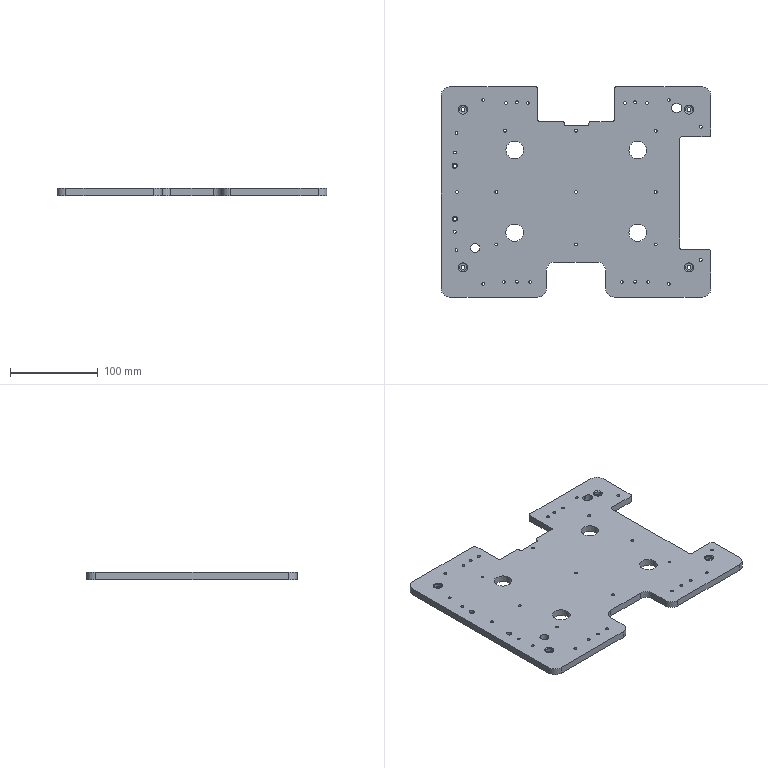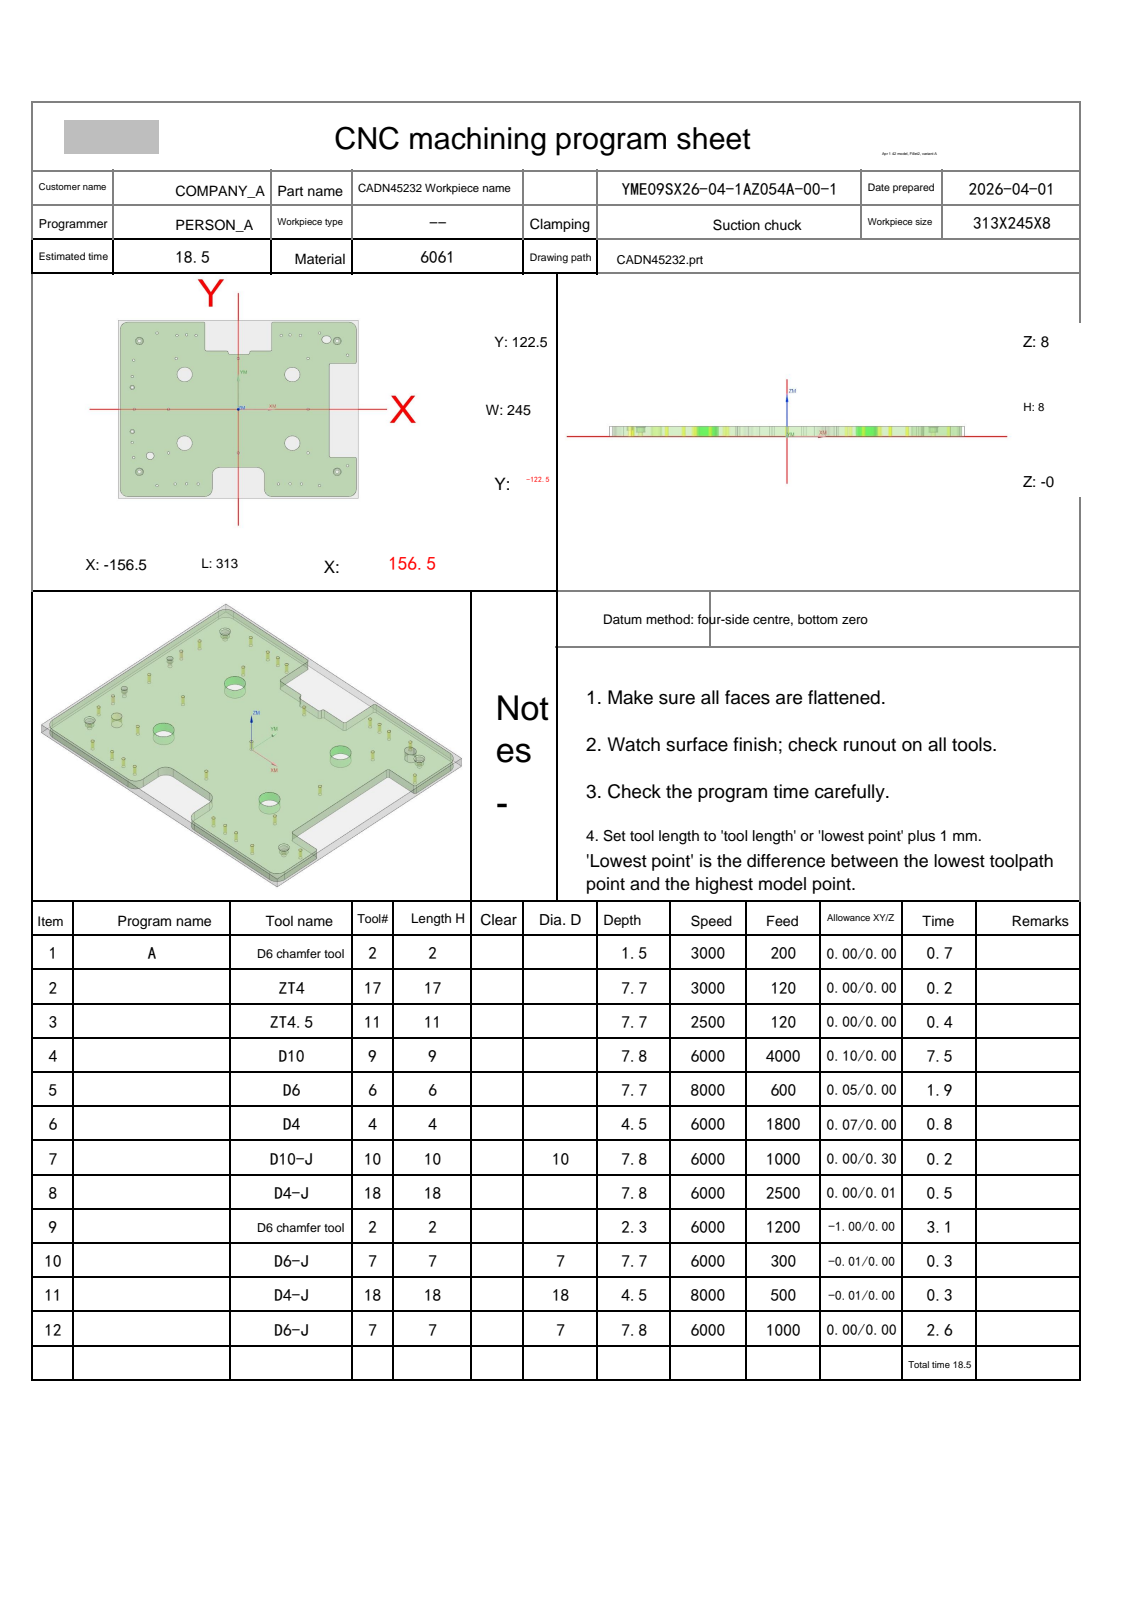NC program | NX | posted by the shop | part box 308 x 240 x 8 mm
Lines 6151 to 6786 of 6786:
N9 T02 M06
(D6 chamfer tool  D=6. R=0. H=02 ce=0.00 di=0.00)
G00 G90 G54 X-156.128 Y-.25 M03 S6000
G43 H02 Z28.
M08
Z10.099
G01 Z6.501 F1200.
G03 X-155.828 Y-.33 I.3 J.52
X-155.308 Y-.03 I0.0 J.6
G01 X-155.3 Y0.0
Y110.
G02 X-144. Y121.3 I11.3 J0.0
G01 X-45.5
G02 X-42.2 Y118. I0.0 J-3.3
G01 Y82.355
X-42.178 Y82.137
X-42.117 Y81.965
X-42.002 Y81.806
X-41.848 Y81.685
X-41.666 Y81.612
X-41.435 Y81.589
X-15.216
X-15.151 Y81.587
X-15.087 Y81.582
X-14.647 Y81.538
X-14.491 Y81.513
X-14.34 Y81.469
X-13.846 Y81.293
X-13.678 Y81.219
X-13.522 Y81.123
X-13.063 Y80.793
X-12.923 Y80.675
X-12.8 Y80.539
X-12.451 Y80.094
X-12.349 Y79.942
X-12.269 Y79.777
X-12.058 Y79.253
X-12.002 Y79.078
G02 X-11.909 Y78.005 I-6.16 J-1.074
X-11.916 Y77.706 I-6.252 J0.0
G03 X-11.216 Y77.006 I.7 J0.0
G01 X12.784
G03 X13.484 Y77.706 I0.0 J.7
G02 X13.476 Y78.014 I5.995 J.309
X13.559 Y79.013 I6.003 J0.0
G01 X13.603 Y79.164
X13.779 Y79.659
X13.853 Y79.827
X13.949 Y79.983
X14.28 Y80.441
X14.397 Y80.582
X14.533 Y80.705
X14.978 Y81.053
X15.13 Y81.156
X15.295 Y81.236
X15.819 Y81.447
X15.994 Y81.503
X16.174 Y81.534
X16.654 Y81.582
X16.719 Y81.587
X16.784 Y81.589
X41.435
X41.652 Y81.611
X41.824 Y81.672
X41.983 Y81.786
X42.104 Y81.941
X42.177 Y82.123
X42.2 Y82.355
Y118.
G02 X45.5 Y121.3 I3.3 J0.0
G01 X144.
G02 X155.3 Y110. I0.0 J-11.3
G01 Y65.004
G02 X152. Y61.704 I-3.3 J0.0
G01 X120.728
X120.511 Y61.682
X120.339 Y61.621
X120.18 Y61.506
X120.059 Y61.352
X119.986 Y61.17
X119.963 Y60.939
Y-63.931
X119.984 Y-64.149
X120.046 Y-64.32
X120.16 Y-64.479
X120.315 Y-64.6
X120.497 Y-64.673
X120.728 Y-64.696
X152.
G02 X155.3 Y-67.996 I0.0 J-3.3
G01 Y-110.
G02 X144. Y-121.3 I-11.3 J0.0
G01 X44.
G02 X32.7 Y-110. I0.0 J11.3
G01 Y-90.
G03 X24. Y-81.3 I-8.7 J0.0
G01 X-24.
G03 X-32.7 Y-90. I0.0 J-8.7
G01 Y-110.
G02 X-44. Y-121.3 I-11.3 J0.0
G01 X-144.
G02 X-155.3 Y-110. I0.0 J11.3
G01 Y0.0
X-155.308 Y.03
G03 X-155.828 Y.33 I-.52 J-.3
X-156.128 Y.25 I0.0 J-.6
G01 Z10.099
G00 Z28.
X-77.885 Y48.289
Z10.119
G01 Z6.501
G03 X-78.16 Y48.355 I-.275 J-.533
X-78.693 Y48.03 I0.0 J-.6
G01 X-78.7 Y48.
G03 X-70. Y39.3 I8.7 J0.0
X-61.3 Y48. I0.0 J8.7
X-70. Y56.7 I-8.7 J0.0
X-78.7 Y48. I0.0 J-8.7
G01 X-78.693 Y47.97
G03 X-78.16 Y47.645 I.533 J.275
X-77.885 Y47.711 I0.0 J.6
G01 Z10.119
G00 Z28.
X-77.99 Y-46.278
Z10.119
G01 Z6.501
G03 X-78.265 Y-46.211 I-.275 J-.533
X-78.798 Y-46.536 I0.0 J-.6
G01 X-78.805 Y-46.566
G03 X-70.105 Y-55.266 I8.7 J0.0
X-61.405 Y-46.566 I0.0 J8.7
X-70.105 Y-37.866 I-8.7 J0.0
X-78.805 Y-46.566 I0.0 J-8.7
G01 X-78.798 Y-46.597
G03 X-78.265 Y-46.922 I.533 J.275
X-77.99 Y-46.855 I0.0 J.6
G01 Z10.119
G00 Z28.
X62.573 Y-46.278
Z10.119
G01 Z6.501
G03 X62.298 Y-46.211 I-.275 J-.533
X61.765 Y-46.536 I0.0 J-.6
G01 X61.758 Y-46.566
G03 X70.458 Y-55.266 I8.7 J0.0
X79.158 Y-46.566 I0.0 J8.7
X70.458 Y-37.866 I-8.7 J0.0
X61.758 Y-46.566 I0.0 J-8.7
G01 X61.765 Y-46.597
G03 X62.298 Y-46.922 I.533 J.275
X62.573 Y-46.855 I0.0 J.6
G01 Z10.119
G00 Z28.
Y48.135
Z10.119
G01 Z6.501
G03 X62.298 Y48.202 I-.275 J-.533
X61.765 Y47.877 I0.0 J-.6
G01 X61.758 Y47.847
G03 X70.458 Y39.147 I8.7 J0.0
X79.158 Y47.847 I0.0 J8.7
X70.458 Y56.547 I-8.7 J0.0
X61.758 Y47.847 I0.0 J-8.7
G01 X61.765 Y47.816
G03 X62.298 Y47.491 I.533 J.275
X62.573 Y47.558 I0.0 J.6
G01 Z10.119
G00 Z28.
X114.75 Y93.136
Z10.099
G01 Z6.501
G03 X114.67 Y92.836 I.52 J-.3
X114.97 Y92.317 I.6 J0.0
G01 X115. Y92.309
X116.
G03 X119.7 Y96.009 I0.0 J3.7
X116. Y99.709 I-3.7 J0.0
G01 X114.
G03 X110.3 Y96.009 I0.0 J-3.7
X114. Y92.309 I3.7 J0.0
G01 X115.
X115.03 Y92.317
G03 X115.33 Y92.836 I-.3 J.52
X115.25 Y93.136 I-.6 J0.0
G01 Z10.099
G00 Z28.
G00 G90 X0.0 Y0.0 M03 S5000
Z28.
G98 G81 X0.0 Y0.0 Z5.8 R11. F150.
Y-60.
X-52.35 Y-102.765
X-67.5 Y-102.5
X-82.35 Y-102.765
X-106. Y-105.
X-136.5 Y-66.5
X-138.327 Y-45.597
X-91. Y-60.
Y0.0
X-135.8
X-138.327 Y45.083
X-136.5 Y67.5
X-106. Y105.
X-81. Y70.
X-80. Y101.6
X-67.5 Y102.5
X-55. Y101.6
X0.0 Y70.
X56. Y101.6
X67.5 Y102.5
X81. Y101.6
X106. Y105.
X142.5 Y74.508
X91. Y70.
Y0.0
Y-60.
X142.5 Y-77.5
X106. Y-105.
X82.35 Y-102.765
X67.5 Y-102.5
X52.35 Y-102.765
G80
G00 Z28.
G00 G90 X-138.239 Y29.77 M03 S6000
Z28.
Z6.5
G01 Z6. F600.
X-138.103 Y29.755
X-137.947 Y29.747
G03 X-137.002 Y30.083 I0.0 J1.5
X-138.327 Y31.408 I-1.325 J0.0
X-139.652 Y30.083 I0.0 J-1.325
X-138.327 Y28.758 I1.325 J0.0
X-137.002 Y30.083 I0.0 J1.325
X-137.947 Y30.418 I-.945 J-1.165
G01 X-138.103 Y30.41
X-138.239 Y30.396
Z6.5
G00 Z28.
Y-30.91
Z6.5
G01 Z6.
X-138.103 Y-30.925
X-137.947 Y-30.933
G03 X-137.002 Y-30.597 I0.0 J1.5
X-138.327 Y-29.272 I-1.325 J0.0
X-139.652 Y-30.597 I0.0 J-1.325
X-138.327 Y-31.922 I1.325 J0.0
X-137.002 Y-30.597 I0.0 J1.325
X-137.947 Y-30.262 I-.945 J-1.165
G01 X-138.103 Y-30.27
X-138.239 Y-30.284
Z6.5
G00 Z28.
G00 G90 X-129.667 Y96.677 M03 S6000
Z28.
Z7.
G01 Z6.5 F600.
X-129.75 Y97.009
G03 X-132.75 Y94.009 I0.0 J-3.
X-129. Y90.259 I3.75 J0.0
X-125.25 Y94.009 I0.0 J3.75
X-129. Y97.759 I-3.75 J0.0
X-132.75 Y94.009 I0.0 J-3.75
X-129.75 Y91.009 I3. J0.0
G01 X-129.667 Y91.341
Z7.
G00 Z28.
Y-83.323
Z7.
G01 Z6.5
X-129.75 Y-82.991
G03 X-132.75 Y-85.991 I0.0 J-3.
X-129. Y-89.741 I3.75 J0.0
X-125.25 Y-85.991 I0.0 J3.75
X-129. Y-82.241 I-3.75 J0.0
X-132.75 Y-85.991 I0.0 J-3.75
X-129.75 Y-88.991 I3. J0.0
G01 X-129.667 Y-88.659
Z7.
G00 Z28.
X128.333 Y-83.323
Z7.
G01 Z6.5
X128.25 Y-82.991
G03 X125.25 Y-85.991 I0.0 J-3.
X129. Y-89.741 I3.75 J0.0
X132.75 Y-85.991 I0.0 J3.75
X129. Y-82.241 I-3.75 J0.0
X125.25 Y-85.991 I0.0 J-3.75
X128.25 Y-88.991 I3. J0.0
G01 X128.333 Y-88.659
Z7.
G00 Z28.
Y96.677
Z7.
G01 Z6.5
X128.25 Y97.009
G03 X125.25 Y94.009 I0.0 J-3.
X129. Y90.259 I3.75 J0.0
X132.75 Y94.009 I0.0 J3.75
X129. Y97.759 I-3.75 J0.0
X125.25 Y94.009 I0.0 J-3.75
X128.25 Y91.009 I3. J0.0
G01 X128.333 Y91.341
Z7.
G00 Z28.
G00 G90 X-115.034 Y-61.942 M03 S6000
Z28.
Z6.2
G01 Z5.7 F600.
X-115.05 Y-60.991
G03 X-118.05 Y-63.991 I0.0 J-3.
X-115. Y-67.041 I3.05 J0.0
X-111.95 Y-63.991 I0.0 J3.05
X-115. Y-60.941 I-3.05 J0.0
X-118.05 Y-63.991 I0.0 J-3.05
X-115.05 Y-66.991 I3. J0.0
G01 X-115.034 Y-66.041
Z6.2
G00 Z28.
G91 G28 Z0.0
M05
M09
G91 G28 Z0.0
M01
N10 T07 M06
(D6-J  D=6. R=0. H=07 ce=-0.01 di=0.00)
G00 G90 G54 X115.2 Y97.769 M03 S6000
G43 H07 Z28.
M08
Z4.651
G01 Z4.151 F300.
G41 D07
Y97.819
G03 X115. Y98.019 I-.2 J0.0
G01 X114.
G03 X111.99 Y96.009 I0.0 J-2.01
X114. Y93.999 I2.01 J0.0
G01 X116.
G03 X118.01 Y96.009 I0.0 J2.01
X116. Y98.019 I-2.01 J0.0
G01 X115.
X114.5
G03 X114.3 Y97.819 I0.0 J-.2
G01 G40 Y97.769
Z4.651
G00 Z8.5
X115.2
Z.803
G01 Z.303
G41 D07
Y97.819
G03 X115. Y98.019 I-.2 J0.0
G01 X114.
G03 X111.99 Y96.009 I0.0 J-2.01
X114. Y93.999 I2.01 J0.0
G01 X116.
G03 X118.01 Y96.009 I0.0 J2.01
X116. Y98.019 I-2.01 J0.0
G01 X115.
X114.5
G03 X114.3 Y97.819 I0.0 J-.2
G01 G40 Y97.769
Z.803
G00 Z28.
X-116.799 Y-63.791
Z4.651
G01 Z4.151
G41 D07
X-116.86
G03 X-117.06 Y-63.991 I0.0 J-.2
X-115. Y-66.051 I2.06 J0.0
X-112.94 Y-63.991 I0.0 J2.06
X-115. Y-61.931 I-2.06 J0.0
X-117.06 Y-63.991 I0.0 J-2.06
X-117. Y-64.486 I2.06 J0.0
X-116.805 Y-64.639 I.194 J.048
G01 X-116.747 Y-64.63
G40 X-116.698 Y-64.618
Z4.651
G00 Z8.5
X-116.799 Y-63.791
Z.803
G01 Z.303
G41 D07
X-116.86
G03 X-117.06 Y-63.991 I0.0 J-.2
X-115. Y-66.051 I2.06 J0.0
X-112.94 Y-63.991 I0.0 J2.06
X-115. Y-61.931 I-2.06 J0.0
X-117.06 Y-63.991 I0.0 J-2.06
X-117. Y-64.486 I2.06 J0.0
X-116.805 Y-64.639 I.194 J.048
G01 X-116.747 Y-64.63
G40 X-116.698 Y-64.618
Z.803
G00 Z28.
G91 G28 Z0.0
M05
M09
G91 G28 Z0.0
M01
N11 T18 M06
(D4-J  D=4. R=0. H=18 ce=-0.01 di=0.00)
G00 G90 G54 X-130.021 Y94.809 M03 S8000
G43 H18 Z19.5
M08
Z4.5
G01 Z3.5 F500.
G41 D18
X-130.46
G03 X-131.26 Y94.009 I0.0 J-.8
X-129. Y91.749 I2.26 J0.0
X-126.74 Y94.009 I0.0 J2.26
X-129. Y96.269 I-2.26 J0.0
X-131.26 Y94.009 I0.0 J-2.26
X-131.225 Y93.611 I2.26 J0.0
X-130.437 Y92.952 I.788 J.141
G01 X-130.296 Y92.964
X-130.061 Y93.006
G40 X-129.865 Y93.041
Z4.5
G00 Z19.5
X-138.394 Y30.308
Z6.
G01 Z5.
G41 D18
X-138.562 Y30.883
G03 X-139.362 Y30.083 I0.0 J-.8
X-138.327 Y29.048 I1.035 J0.0
X-137.292 Y30.083 I0.0 J1.035
X-138.327 Y31.118 I-1.035 J0.0
X-139.362 Y30.083 I0.0 J-1.035
X-139.286 Y29.693 I1.035 J0.0
X-138.545 Y29.194 I.741 J.302
X-138.243 Y29.253 I0.0 J.8
G01 G40 X-138.304 Y29.849
Z6.
G00 Z19.5
X-138.394 Y-30.372
Z6.
G01 Z5.
G41 D18
X-138.562 Y-29.797
G03 X-139.362 Y-30.597 I0.0 J-.8
X-138.327 Y-31.632 I1.035 J0.0
X-137.292 Y-30.597 I0.0 J1.035
X-138.327 Y-29.562 I-1.035 J0.0
X-139.362 Y-30.597 I0.0 J-1.035
X-139.286 Y-30.987 I1.035 J0.0
X-138.545 Y-31.486 I.741 J.302
X-138.243 Y-31.427 I0.0 J.8
G01 G40 X-138.304 Y-30.831
Z6.
G00 Z19.5
X-130.021 Y-85.191
Z4.5
G01 Z3.5
G41 D18
X-130.46
G03 X-131.26 Y-85.991 I0.0 J-.8
X-129. Y-88.251 I2.26 J0.0
X-126.74 Y-85.991 I0.0 J2.26
X-129. Y-83.731 I-2.26 J0.0
X-131.26 Y-85.991 I0.0 J-2.26
X-131.225 Y-86.389 I2.26 J0.0
X-130.437 Y-87.048 I.788 J.141
G01 X-130.296 Y-87.036
X-130.061 Y-86.994
G40 X-129.865 Y-86.959
Z4.5
G00 Z19.5
X130.021 Y-86.791
Z4.5
G01 Z3.5
G41 D18
X130.46
G03 X131.26 Y-85.991 I0.0 J.8
X129. Y-83.731 I-2.26 J0.0
X126.74 Y-85.991 I0.0 J-2.26
X129. Y-88.251 I2.26 J0.0
X131.26 Y-85.991 I0.0 J2.26
X131.225 Y-85.593 I-2.26 J0.0
X130.437 Y-84.934 I-.788 J-.141
G01 X130.296 Y-84.947
X130.061 Y-84.989
G40 X129.865 Y-85.024
Z4.5
G00 Z19.5
X130.021 Y93.209
Z4.5
G01 Z3.5
G41 D18
X130.46
G03 X131.26 Y94.009 I0.0 J.8
X129. Y96.269 I-2.26 J0.0
X126.74 Y94.009 I0.0 J-2.26
X129. Y91.749 I2.26 J0.0
X131.26 Y94.009 I0.0 J2.26
X131.225 Y94.407 I-2.26 J0.0
X130.437 Y95.066 I-.788 J-.141
G01 X130.296 Y95.053
X130.061 Y95.011
G40 X129.865 Y94.976
Z4.5
G00 Z19.5
G91 G28 Z0.0
M05
M09
G91 G28 Z0.0
M01
N12 T07 M06
(D6-J  D=6. R=0. H=07 ce=0.00 di=0.00)
G00 G90 G54 X-158.164 Y-111.007 M03 S6000
G43 H07 Z28.
M08
Z1.
G01 Z.5 F1000.
G41 D07
X-157.964 Y-110.999
G03 X-157. Y-110. I-.036 J.999
G01 Y110.
G02 X-144. Y123. I13. J0.0
G01 X-45.5
G02 X-40.5 Y118. I0.0 J-5.
G01 Y83.289
X-15.066
X-14.22 Y83.204
X-13.263 Y82.908
X-12.384 Y82.427
X-11.618 Y81.782
X-10.995 Y80.997
X-10.541 Y80.104
X-10.28 Y79.16
X-10.241 Y78.706
X11.811
X11.869 Y79.285
X12.165 Y80.242
X12.645 Y81.12
X13.29 Y81.887
X14.075 Y82.509
X14.968 Y82.963
X15.911 Y83.225
X16.656 Y83.289
X40.5
Y118.
G02 X45.5 Y123. I5. J0.0
G01 X144.
G02 X157. Y110. I0.0 J-13.
G01 Y65.004
G02 X152. Y60.004 I-5. J0.0
G01 X121.663
Y-62.996
X152.
G02 X157. Y-67.996 I0.0 J-5.
G01 Y-110.
G02 X144. Y-123. I-13. J0.0
G01 X44.
G02 X31. Y-110. I0.0 J13.
G01 Y-90.
G03 X24. Y-83. I-7. J0.0
G01 X-24.
G03 X-31. Y-90. I0.0 J-7.
G01 Y-110.
G02 X-44. Y-123. I-13. J0.0
G01 X-144.
G02 X-157. Y-110. I0.0 J13.
G01 Y-109.5
G03 X-158. Y-108.5 I-1. J0.0
G01 G40 X-158.2
Z1.
G00 Z28.
G00 G90 X-158.064 Y-111.003 M03 S6000
Z28.
Z.7
G01 Z.2 F1000.
G41 D07
X-157.964 Y-110.999
G03 X-157. Y-110. I-.036 J.999
G01 Y110.
G02 X-144. Y123. I13. J0.0
G01 X-45.5
G02 X-40.5 Y118. I0.0 J-5.
G01 Y83.289
X-15.066
X-14.22 Y83.204
X-13.263 Y82.908
X-12.384 Y82.427
X-11.618 Y81.782
X-10.995 Y80.997
X-10.541 Y80.104
X-10.28 Y79.16
X-10.241 Y78.706
X11.811
X11.869 Y79.285
X12.165 Y80.242
X12.645 Y81.12
X13.29 Y81.887
X14.075 Y82.509
X14.968 Y82.963
X15.911 Y83.225
X16.656 Y83.289
X40.5
Y118.
G02 X45.5 Y123. I5. J0.0
G01 X144.
G02 X157. Y110. I0.0 J-13.
G01 Y65.004
G02 X152. Y60.004 I-5. J0.0
G01 X121.663
Y-62.996
X152.
G02 X157. Y-67.996 I0.0 J-5.
G01 Y-110.
G02 X144. Y-123. I-13. J0.0
G01 X44.
G02 X31. Y-110. I0.0 J13.
G01 Y-90.
G03 X24. Y-83. I-7. J0.0
G01 X-24.
G03 X-31. Y-90. I0.0 J-7.
G01 Y-110.
G02 X-44. Y-123. I-13. J0.0
G01 X-144.
G02 X-157. Y-110. I0.0 J13.
G01 Y-109.5
G03 X-158. Y-108.5 I-1. J0.0
G01 G40 X-158.1
Z.7
G00 Z28.
M05
M09
G91 G28 Z0.0
G91 G28 Y0.0
M30
%